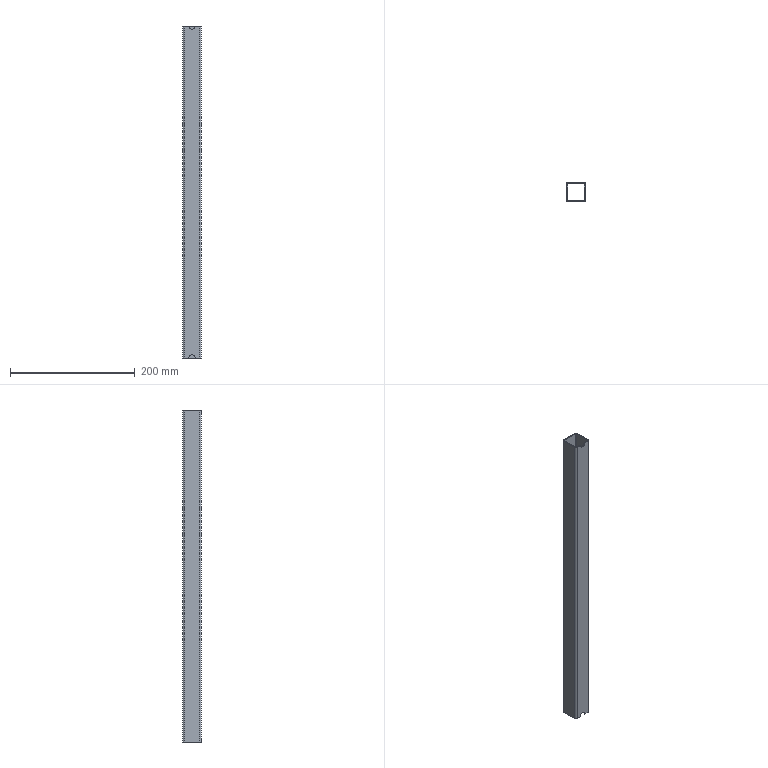Part | STEP file | PN_0043_default | 1 solid | 20 faces | box 30 x 30 x 532 mm | volume 88457 mm3 | plane 10 | cylinder 10 | commonest cylinder face diameters 2 x4 5 x4 10 x2